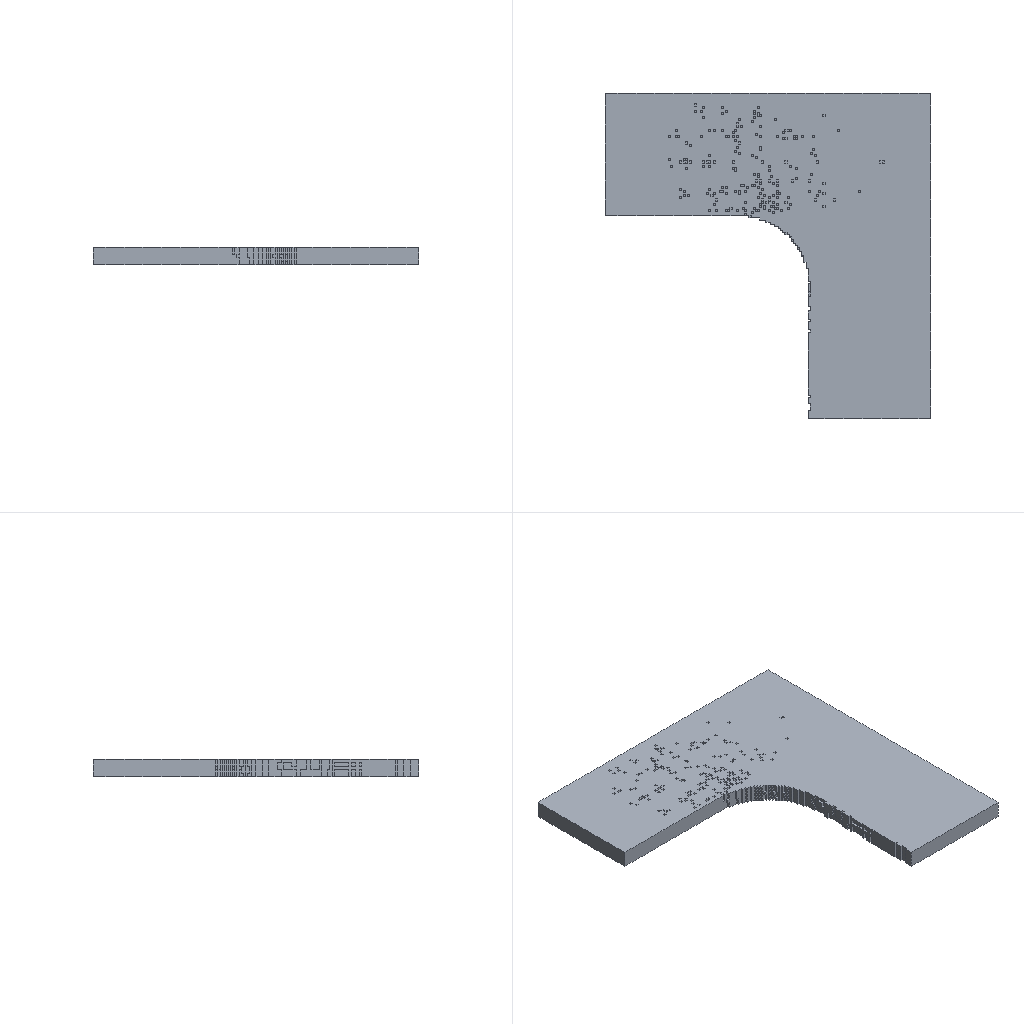Simulation study | abaqus
Set-up summary:
category,name,step,type,value,unit,region
solver,abaqus
solver,version,,,Abaqus/Explicit 2020
units,not stated in the deck,,not stated
analysis,deck,,transient,transient
load_step,Step-1,Step-1,transient
load_step,requested,,,1
mesh,nodes,,,180188
mesh,elements,,,145030
element_type,SC8R,,solid_shell,145030
load,load commands in deck,,count,1
bc,support commands in deck,,count,2
material,MATERIAL-1,,in results
check,setup vs results,,match,"per instance, exact: element labels, types and connectivity; labels of the nodes the elements use; coordinates not compared"
Abaqus input file, long lists of numbers shortened:
*Heading
** Job name: Job-1 Model name: L
** Generated by: Abaqus/CAE 2020
*Preprint, echo=NO, model=NO, history=NO, contact=NO
**
** PARTS
**
*Part, name=PART-1
*Node
      1,   1.216,   74.944,       -0.625
      2,   1.216,    75.712,       -0.625
** (90092 more lines like these left out)
*Element, type=SC8R
    1, 14845, 15000, 15001, 14846, 29846, 30001, 30002, 29847
    2, 14690, 14845, 14846, 14691, 29691, 29846, 29847, 29692
** (72513 more lines like these left out)
*Elset, elset=Set-3, generate
     1,  72515,      1
*Orientation, name=Ori-1
1., 0., 0., 0., 1., 0.
1, 0.
** Section: Section-1
*Shell Section, elset=Set-3, material=Material-1, orientation=Ori-1
5., 5
*End Part
**
**
** ASSEMBLY
**
*Assembly, name=Assembly
**
*Instance, name=PART-1-1, part=PART-1
*End Instance
**
*Instance, name=PART-1-2, part=PART-1
*End Instance
**
*Node
      1,   1.216,   119.488,        1.875
*Nset, nset=Set-4, instance=PART-1-1
 12677, 12678, 12832, 12833, 12834, 12987, 12988, 12989, 12990, 12991, 13142, 13143, 13144, 13145, 13146, 13147
 13297, 13298, 13299, 13300, 13301, 13302, 13303, 13304, 13452, 13453, 13454, 13455, 13456, 13457, 13458, 13459
** (69 more lines like these left out)
*Nset, nset=Set-4, instance=PART-1-2
 12677, 12678, 12832, 12833, 12834, 12987, 12988, 12989, 12990, 12991, 13142, 13143, 13144, 13145, 13146, 13147
 13297, 13298, 13299, 13300, 13301, 13302, 13303, 13304, 13452, 13453, 13454, 13455, 13456, 13457, 13458, 13459
** (69 more lines like these left out)
*Nset, nset=Set-5, instance=PART-1-1
    46,    47,    48,    49,    50,    51,    52,    53,    54,    55,    56,    57,    58,    59,   105,   106
   107,   108,   109,   110,   111,   112,   113,   114,   115,   116,   117,   118,   165,   166,   167,   168
** (57 more lines like these left out)
*Nset, nset=Set-5, instance=PART-1-2
    46,    47,    48,    49,    50,    51,    52,    53,    54,    55,    56,    57,    58,    59,   105,   106
   107,   108,   109,   110,   111,   112,   113,   114,   115,   116,   117,   118,   165,   166,   167,   168
** (57 more lines like these left out)
*Nset, nset=Set-GD, instance=PART-1-1
  6012,  6167,  6168,  6322,  6323,  6324,  6477,  6478,  6479,  6480,  6632,  6633,  6634,  6635,  6636,  6787
  6788,  6789,  6790,  6791,  6792,  6942,  6943,  6944,  6945,  6946,  6947,  6948,  7097,  7098,  7099,  7100
** (659 more lines like these left out)
*Nset, nset=Set-GD, instance=PART-1-2
  6012,  6167,  6168,  6322,  6323,  6324,  6477,  6478,  6479,  6480,  6632,  6633,  6634,  6635,  6636,  6787
  6788,  6789,  6790,  6791,  6792,  6942,  6943,  6944,  6945,  6946,  6947,  6948,  7097,  7098,  7099,  7100
** (659 more lines like these left out)
*Nset, nset=Set-NODE, instance=PART-1-1
     3,     4,     5,     6,     7,     8,     9,    10,    11,    12,    13,    14,    15,    16,    17,    18
    19,    20,    21,    22,    23,    24,    25,    26,    27,    28,    29,    30,    31,    32,    33,    34
** (633 more lines like these left out)
*Nset, nset=Set-NODE, instance=PART-1-2
     3,     4,     5,     6,     7,     8,     9,    10,    11,    12,    13,    14,    15,    16,    17,    18
    19,    20,    21,    22,    23,    24,    25,    26,    27,    28,    29,    30,    31,    32,    33,    34
** (633 more lines like these left out)
*Nset, nset=Set-PR
 1,
*Nset, nset="_T-Datum csys-1", internal
Set-5,
*Transform, nset="_T-Datum csys-1"
-0.7071, 0.7071,           0., 0.7071, 0.7071,           0.
*End Assembly
**
** MATERIALS
**
*Material, name=Material-1
*Damage Initiation, criterion=HASHIN
1518.,657., 29.,136., 67., 67.
*Damage Evolution, type=ENERGY
 2e+08, 2e+08, 2e+08, 2e+08
*Damage Stabilization
0.001,0.001,0.001,0.001
*Density
 2e-09,
*Elastic, type=ENGINEERING CONSTANTS
54000.,54000.,54000.,  0.25,  0.35,  0.35,16000.,24000.
24000.,
** ----------------------------------------------------------------
**
** STEP: Step-1
**
*Step, name=Step-1, nlgeom=YES
*Dynamic, Explicit
, 1.
*Bulk Viscosity
0.06, 1.2
** Mass Scaling: Semi-Automatic
**               Whole Model
*Fixed Mass Scaling, factor=500.
**
** BOUNDARY CONDITIONS
**
** Name: BC-1 Type: 对称/反对称/完全固定
*Boundary
Set-4, ENCASTRE
** Name: BC-2 Type: 速度/角速度
*Boundary, type=VELOCITY
Set-5, 1, 1, 1.
**
** OUTPUT REQUESTS
**
*Restart, write, number interval=1, time marks=NO
**
** FIELD OUTPUT: F-Output-1
**
*Output, field, number interval=500, time marks=YES
*Node Output
RF, U, V
*Element Output, directions=YES
DAMAGEC, DAMAGEFC, DAMAGEFT, DAMAGET, E, MISES, PE, PEEQ, PEEQT, PEMAG, PEVAVG, S, SDEG, STATUS, VE, VEEQ
*Contact Output
CSDMG, CSTRESS
*Output, history, frequency=0
*End Step
Results summary:
result,step,Step-1,partial,increments=3320 time=0.006893/1.0
result,analysis,,,transient
result,last_loadstep,,,1
result,primary field,,,U
result,reaction total,,FX,27.163,model units
result,reaction total,,FY,-32.309,model units
result,reaction total,,FZ,0.7949,model units